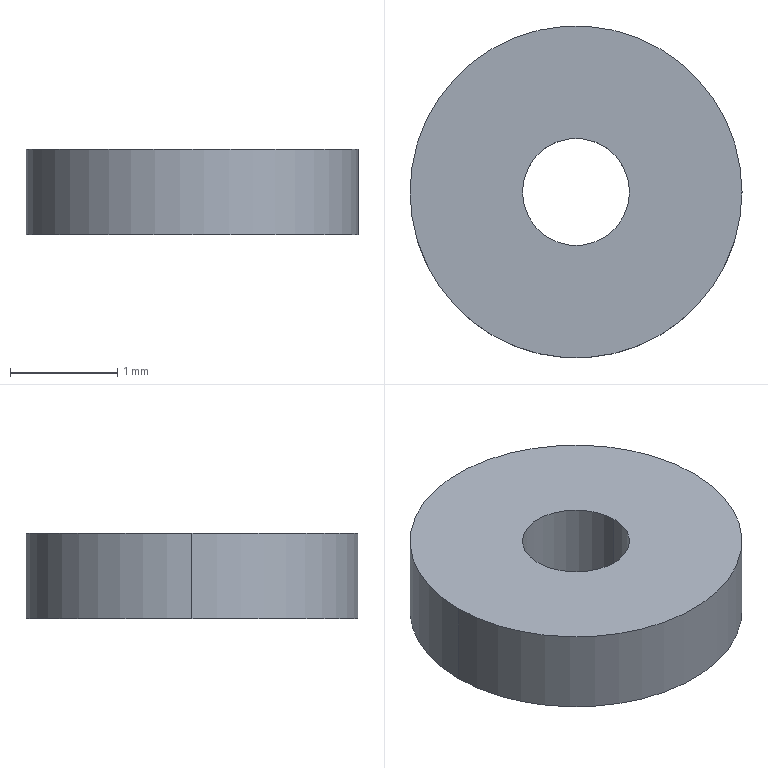Part | STEP file | 05-04 bending roller | 1 solid | 6 faces | box 3.1 x 3.1 x 0.8 mm | volume 5.41 mm3 | cylinder 4 | plane 2 | commonest cylinder face diameters 1 x2 3.1 x2
STEP:
#1=CARTESIAN_POINT('',(-0.5,0.,0.8));
#2=VERTEX_POINT('',#1);
#3=CARTESIAN_POINT('',(0.5,0.,0.8));
#4=VERTEX_POINT('',#3);
#5=CARTESIAN_POINT('',(0.,0.,0.8));
#6=DIRECTION('',(0.,0.,1.));
#7=DIRECTION('',(1.,0.,0.));
#8=AXIS2_PLACEMENT_3D('',#5,#6,#7);
#9=CIRCLE('',#8,0.5);
#10=EDGE_CURVE('',#2,#4,#9,.T.);
#11=ORIENTED_EDGE('',*,*,#10,.T.);
#12=CARTESIAN_POINT('',(0.5,0.,0.));
#13=VERTEX_POINT('',#12);
#14=CARTESIAN_POINT('',(0.5,0.,0.8));
#15=DIRECTION('',(0.,0.,-1.));
#16=VECTOR('',#15,1000.);
#17=LINE('',#14,#16);
#18=EDGE_CURVE('',#4,#13,#17,.T.);
#19=ORIENTED_EDGE('',*,*,#18,.T.);
#20=CARTESIAN_POINT('',(-0.5,0.,0.));
#21=VERTEX_POINT('',#20);
#22=CARTESIAN_POINT('',(0.,0.,0.));
#23=DIRECTION('',(0.,0.,1.));
#24=DIRECTION('',(1.,0.,0.));
#25=AXIS2_PLACEMENT_3D('',#22,#23,#24);
#26=CIRCLE('',#25,0.5);
#27=EDGE_CURVE('',#21,#13,#26,.T.);
#28=ORIENTED_EDGE('',*,*,#27,.F.);
#29=CARTESIAN_POINT('',(-0.5,0.,0.8));
#30=DIRECTION('',(0.,0.,-1.));
#31=VECTOR('',#30,1000.);
#32=LINE('',#29,#31);
#33=EDGE_CURVE('',#2,#21,#32,.T.);
#34=ORIENTED_EDGE('',*,*,#33,.F.);
#35=EDGE_LOOP('',(#11,#19,#28,#34));
#36=FACE_OUTER_BOUND('',#35,.T.);
#37=CARTESIAN_POINT('',(0.,0.,0.8));
#38=DIRECTION('',(0.,0.,-1.));
#39=DIRECTION('',(-1.,0.,0.));
#40=AXIS2_PLACEMENT_3D('',#37,#38,#39);
#41=CYLINDRICAL_SURFACE('',#40,0.5);
#42=ADVANCED_FACE('',(#36),#41,.F.);
#43=CARTESIAN_POINT('',(1.55,0.,0.8));
#44=VERTEX_POINT('',#43);
#45=CARTESIAN_POINT('',(-1.55,0.,0.8));
#46=VERTEX_POINT('',#45);
#47=CARTESIAN_POINT('',(0.,0.,0.8));
#48=DIRECTION('',(0.,0.,1.));
#49=DIRECTION('',(1.,0.,0.));
#50=AXIS2_PLACEMENT_3D('',#47,#48,#49);
#51=CIRCLE('',#50,1.55);
#52=EDGE_CURVE('',#44,#46,#51,.T.);
#53=ORIENTED_EDGE('',*,*,#52,.F.);
#54=CARTESIAN_POINT('',(1.55,0.,0.));
#55=VERTEX_POINT('',#54);
#56=CARTESIAN_POINT('',(1.55,0.,0.8));
#57=DIRECTION('',(0.,0.,-1.));
#58=VECTOR('',#57,1000.);
#59=LINE('',#56,#58);
#60=EDGE_CURVE('',#44,#55,#59,.T.);
#61=ORIENTED_EDGE('',*,*,#60,.T.);
#62=CARTESIAN_POINT('',(-1.55,0.,0.));
#63=VERTEX_POINT('',#62);
#64=CARTESIAN_POINT('',(0.,0.,0.));
#65=DIRECTION('',(0.,0.,1.));
#66=DIRECTION('',(1.,0.,0.));
#67=AXIS2_PLACEMENT_3D('',#64,#65,#66);
#68=CIRCLE('',#67,1.55);
#69=EDGE_CURVE('',#55,#63,#68,.T.);
#70=ORIENTED_EDGE('',*,*,#69,.T.);
#71=CARTESIAN_POINT('',(-1.55,0.,0.8));
#72=DIRECTION('',(0.,0.,-1.));
#73=VECTOR('',#72,1000.);
#74=LINE('',#71,#73);
#75=EDGE_CURVE('',#46,#63,#74,.T.);
#76=ORIENTED_EDGE('',*,*,#75,.F.);
#77=EDGE_LOOP('',(#53,#61,#70,#76));
#78=FACE_OUTER_BOUND('',#77,.T.);
#79=CARTESIAN_POINT('',(0.,0.,0.8));
#80=DIRECTION('',(0.,0.,-1.));
#81=DIRECTION('',(-1.,0.,0.));
#82=AXIS2_PLACEMENT_3D('',#79,#80,#81);
#83=CYLINDRICAL_SURFACE('',#82,1.55);
#84=ADVANCED_FACE('',(#78),#83,.T.);
#85=CARTESIAN_POINT('',(0.,0.,0.8));
#86=DIRECTION('',(0.,0.,1.));
#87=DIRECTION('',(1.,0.,0.));
#88=AXIS2_PLACEMENT_3D('',#85,#86,#87);
#89=CIRCLE('',#88,1.55);
#90=EDGE_CURVE('',#46,#44,#89,.T.);
#91=ORIENTED_EDGE('',*,*,#90,.T.);
#92=ORIENTED_EDGE('',*,*,#52,.T.);
#93=EDGE_LOOP('',(#91,#92));
#94=FACE_OUTER_BOUND('',#93,.T.);
#95=ORIENTED_EDGE('',*,*,#10,.F.);
#96=CARTESIAN_POINT('',(0.,0.,0.8));
#97=DIRECTION('',(0.,0.,1.));
#98=DIRECTION('',(1.,0.,0.));
#99=AXIS2_PLACEMENT_3D('',#96,#97,#98);
#100=CIRCLE('',#99,0.5);
#101=EDGE_CURVE('',#4,#2,#100,.T.);
#102=ORIENTED_EDGE('',*,*,#101,.F.);
#103=EDGE_LOOP('',(#95,#102));
#104=FACE_BOUND('',#103,.T.);
#105=CARTESIAN_POINT('',(0.,0.,0.8));
#106=DIRECTION('',(0.,0.,1.));
#107=DIRECTION('',(1.,0.,0.));
#108=AXIS2_PLACEMENT_3D('',#105,#106,#107);
#109=PLANE('',#108);
#110=ADVANCED_FACE('',(#94,#104),#109,.T.);
#111=CARTESIAN_POINT('',(0.,0.,0.));
#112=DIRECTION('',(0.,0.,1.));
#113=DIRECTION('',(1.,0.,0.));
#114=AXIS2_PLACEMENT_3D('',#111,#112,#113);
#115=CIRCLE('',#114,1.55);
#116=EDGE_CURVE('',#63,#55,#115,.T.);
#117=ORIENTED_EDGE('',*,*,#116,.F.);
#118=ORIENTED_EDGE('',*,*,#69,.F.);
#119=EDGE_LOOP('',(#117,#118));
#120=FACE_OUTER_BOUND('',#119,.T.);
#121=ORIENTED_EDGE('',*,*,#27,.T.);
#122=CARTESIAN_POINT('',(0.,0.,0.));
#123=DIRECTION('',(0.,0.,1.));
#124=DIRECTION('',(1.,0.,0.));
#125=AXIS2_PLACEMENT_3D('',#122,#123,#124);
#126=CIRCLE('',#125,0.5);
#127=EDGE_CURVE('',#13,#21,#126,.T.);
#128=ORIENTED_EDGE('',*,*,#127,.T.);
#129=EDGE_LOOP('',(#121,#128));
#130=FACE_BOUND('',#129,.T.);
#131=CARTESIAN_POINT('',(0.,0.,0.));
#132=DIRECTION('',(0.,0.,1.));
#133=DIRECTION('',(1.,0.,0.));
#134=AXIS2_PLACEMENT_3D('',#131,#132,#133);
#135=PLANE('',#134);
#136=ADVANCED_FACE('',(#120,#130),#135,.F.);
#137=ORIENTED_EDGE('',*,*,#60,.F.);
#138=ORIENTED_EDGE('',*,*,#90,.F.);
#139=ORIENTED_EDGE('',*,*,#75,.T.);
#140=ORIENTED_EDGE('',*,*,#116,.T.);
#141=EDGE_LOOP('',(#137,#138,#139,#140));
#142=FACE_OUTER_BOUND('',#141,.T.);
#143=CARTESIAN_POINT('',(0.,0.,0.8));
#144=DIRECTION('',(0.,0.,-1.));
#145=DIRECTION('',(-1.,0.,0.));
#146=AXIS2_PLACEMENT_3D('',#143,#144,#145);
#147=CYLINDRICAL_SURFACE('',#146,1.55);
#148=ADVANCED_FACE('',(#142),#147,.T.);
#149=ORIENTED_EDGE('',*,*,#18,.F.);
#150=ORIENTED_EDGE('',*,*,#101,.T.);
#151=ORIENTED_EDGE('',*,*,#33,.T.);
#152=ORIENTED_EDGE('',*,*,#127,.F.);
#153=EDGE_LOOP('',(#149,#150,#151,#152));
#154=FACE_OUTER_BOUND('',#153,.T.);
#155=CARTESIAN_POINT('',(0.,0.,0.8));
#156=DIRECTION('',(0.,0.,-1.));
#157=DIRECTION('',(-1.,0.,0.));
#158=AXIS2_PLACEMENT_3D('',#155,#156,#157);
#159=CYLINDRICAL_SURFACE('',#158,0.5);
#160=ADVANCED_FACE('',(#154),#159,.F.);
#161=CLOSED_SHELL('',(#42,#84,#110,#136,#148,#160));
#162=MANIFOLD_SOLID_BREP('',#161);
#163=CARTESIAN_POINT('',(0.,0.,0.));
#164=DIRECTION('',(0.,0.,1.));
#165=DIRECTION('',(1.,0.,0.));
#166=AXIS2_PLACEMENT_3D('',#163,#164,#165);
#167=(LENGTH_UNIT()NAMED_UNIT(*)SI_UNIT(.MILLI.,.METRE.));
#168=UNCERTAINTY_MEASURE_WITH_UNIT(LENGTH_MEASURE(0.00001),#167,'','');
#169=(NAMED_UNIT(*)PLANE_ANGLE_UNIT()SI_UNIT($,.RADIAN.));
#170=(NAMED_UNIT(*)SI_UNIT($,.STERADIAN.)SOLID_ANGLE_UNIT());
#171=(GEOMETRIC_REPRESENTATION_CONTEXT(3)GLOBAL_UNCERTAINTY_ASSIGNED_CONTEXT((#168))GLOBAL_UNIT_ASSIGNED_CONTEXT((#167,#169,#170))REPRESENTATION_CONTEXT('',''));
#172=ADVANCED_BREP_SHAPE_REPRESENTATION('',(#162,#166),#171);